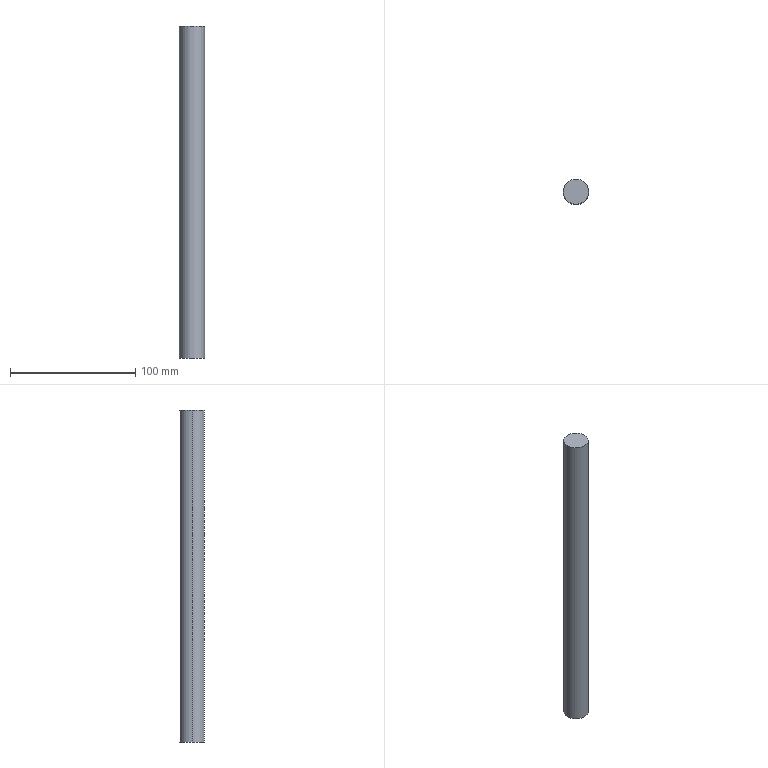Part | SolidWorks | features Extrusion 1 | 1 solid | 4 faces | box 20 x 20 x 265 mm | volume 83252 mm3 | cylinder 2 | plane 2 | commonest cylinder face diameters 20 x2
STEP:
#1=CARTESIAN_POINT('',(10.,0.,265.));
#2=VERTEX_POINT('',#1);
#3=CARTESIAN_POINT('',(-10.,0.,265.));
#4=VERTEX_POINT('',#3);
#5=CARTESIAN_POINT('',(0.,0.,265.));
#6=DIRECTION('',(0.,0.,1.));
#7=DIRECTION('',(1.,0.,0.));
#8=AXIS2_PLACEMENT_3D('',#5,#6,#7);
#9=CIRCLE('',#8,10.);
#10=EDGE_CURVE('',#2,#4,#9,.T.);
#11=ORIENTED_EDGE('',*,*,#10,.F.);
#12=CARTESIAN_POINT('',(10.,0.,0.));
#13=VERTEX_POINT('',#12);
#14=CARTESIAN_POINT('',(10.,0.,265.));
#15=DIRECTION('',(0.,0.,-1.));
#16=VECTOR('',#15,1000.);
#17=LINE('',#14,#16);
#18=EDGE_CURVE('',#2,#13,#17,.T.);
#19=ORIENTED_EDGE('',*,*,#18,.T.);
#20=CARTESIAN_POINT('',(-10.,0.,0.));
#21=VERTEX_POINT('',#20);
#22=CARTESIAN_POINT('',(0.,0.,0.));
#23=DIRECTION('',(0.,0.,1.));
#24=DIRECTION('',(1.,0.,0.));
#25=AXIS2_PLACEMENT_3D('',#22,#23,#24);
#26=CIRCLE('',#25,10.);
#27=EDGE_CURVE('',#13,#21,#26,.T.);
#28=ORIENTED_EDGE('',*,*,#27,.T.);
#29=CARTESIAN_POINT('',(-10.,0.,265.));
#30=DIRECTION('',(0.,0.,-1.));
#31=VECTOR('',#30,1000.);
#32=LINE('',#29,#31);
#33=EDGE_CURVE('',#4,#21,#32,.T.);
#34=ORIENTED_EDGE('',*,*,#33,.F.);
#35=EDGE_LOOP('',(#11,#19,#28,#34));
#36=FACE_OUTER_BOUND('',#35,.T.);
#37=CARTESIAN_POINT('',(0.,0.,265.));
#38=DIRECTION('',(0.,0.,-1.));
#39=DIRECTION('',(-1.,0.,0.));
#40=AXIS2_PLACEMENT_3D('',#37,#38,#39);
#41=CYLINDRICAL_SURFACE('',#40,10.);
#42=ADVANCED_FACE('',(#36),#41,.T.);
#43=ORIENTED_EDGE('',*,*,#18,.F.);
#44=CARTESIAN_POINT('',(0.,0.,265.));
#45=DIRECTION('',(0.,0.,1.));
#46=DIRECTION('',(1.,0.,0.));
#47=AXIS2_PLACEMENT_3D('',#44,#45,#46);
#48=CIRCLE('',#47,10.);
#49=EDGE_CURVE('',#4,#2,#48,.T.);
#50=ORIENTED_EDGE('',*,*,#49,.F.);
#51=ORIENTED_EDGE('',*,*,#33,.T.);
#52=CARTESIAN_POINT('',(0.,0.,0.));
#53=DIRECTION('',(0.,0.,1.));
#54=DIRECTION('',(1.,0.,0.));
#55=AXIS2_PLACEMENT_3D('',#52,#53,#54);
#56=CIRCLE('',#55,10.);
#57=EDGE_CURVE('',#21,#13,#56,.T.);
#58=ORIENTED_EDGE('',*,*,#57,.T.);
#59=EDGE_LOOP('',(#43,#50,#51,#58));
#60=FACE_OUTER_BOUND('',#59,.T.);
#61=CARTESIAN_POINT('',(0.,0.,265.));
#62=DIRECTION('',(0.,0.,-1.));
#63=DIRECTION('',(-1.,0.,0.));
#64=AXIS2_PLACEMENT_3D('',#61,#62,#63);
#65=CYLINDRICAL_SURFACE('',#64,10.);
#66=ADVANCED_FACE('',(#60),#65,.T.);
#67=ORIENTED_EDGE('',*,*,#49,.T.);
#68=ORIENTED_EDGE('',*,*,#10,.T.);
#69=EDGE_LOOP('',(#67,#68));
#70=FACE_OUTER_BOUND('',#69,.T.);
#71=CARTESIAN_POINT('',(0.,0.,265.));
#72=DIRECTION('',(0.,0.,1.));
#73=DIRECTION('',(1.,0.,0.));
#74=AXIS2_PLACEMENT_3D('',#71,#72,#73);
#75=PLANE('',#74);
#76=ADVANCED_FACE('',(#70),#75,.T.);
#77=ORIENTED_EDGE('',*,*,#57,.F.);
#78=ORIENTED_EDGE('',*,*,#27,.F.);
#79=EDGE_LOOP('',(#77,#78));
#80=FACE_OUTER_BOUND('',#79,.T.);
#81=CARTESIAN_POINT('',(0.,0.,0.));
#82=DIRECTION('',(0.,0.,1.));
#83=DIRECTION('',(1.,0.,0.));
#84=AXIS2_PLACEMENT_3D('',#81,#82,#83);
#85=PLANE('',#84);
#86=ADVANCED_FACE('',(#80),#85,.F.);
#87=CLOSED_SHELL('',(#42,#66,#76,#86));
#88=MANIFOLD_SOLID_BREP('',#87);
#89=CARTESIAN_POINT('',(0.,0.,0.));
#90=DIRECTION('',(0.,0.,1.));
#91=DIRECTION('',(1.,0.,0.));
#92=AXIS2_PLACEMENT_3D('',#89,#90,#91);
#93=(LENGTH_UNIT()NAMED_UNIT(*)SI_UNIT(.MILLI.,.METRE.));
#94=UNCERTAINTY_MEASURE_WITH_UNIT(LENGTH_MEASURE(0.00001),#93,'','');
#95=(NAMED_UNIT(*)PLANE_ANGLE_UNIT()SI_UNIT($,.RADIAN.));
#96=(NAMED_UNIT(*)SI_UNIT($,.STERADIAN.)SOLID_ANGLE_UNIT());
#97=(GEOMETRIC_REPRESENTATION_CONTEXT(3)GLOBAL_UNCERTAINTY_ASSIGNED_CONTEXT((#94))GLOBAL_UNIT_ASSIGNED_CONTEXT((#93,#95,#96))REPRESENTATION_CONTEXT('',''));
#98=ADVANCED_BREP_SHAPE_REPRESENTATION('',(#88,#92),#97);